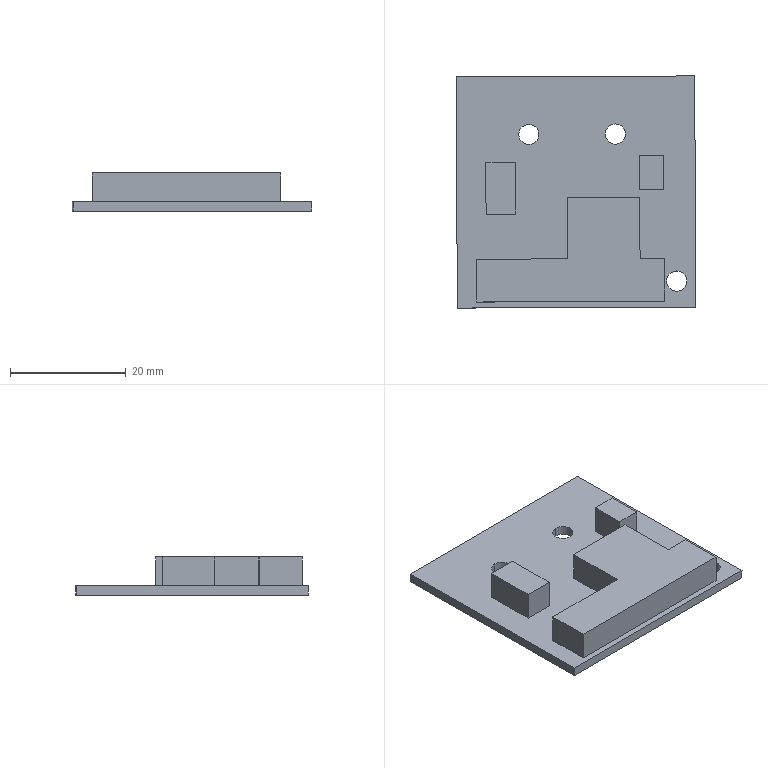Part | SolidWorks | features BaseBody 1 | 1 solid | 31 faces | box 41.444 x 40.179 x 6.6 mm | volume 4823 mm3 | plane 25 | cylinder 6 | commonest cylinder face diameters 3.5 x6
STEP:
#1=CARTESIAN_POINT('',(579.684,-227.507,-73.234));
#2=VERTEX_POINT('',#1);
#3=CARTESIAN_POINT('',(579.684,-224.007,-73.234));
#4=VERTEX_POINT('',#3);
#5=CARTESIAN_POINT('',(579.684,-225.757,-73.234));
#6=DIRECTION('',(-0.000000001,0.000000003,-1.));
#7=DIRECTION('',(0.,-1.,-0.000000003));
#8=AXIS2_PLACEMENT_3D('',#5,#6,#7);
#9=CIRCLE('',#8,1.75);
#10=EDGE_CURVE('',#2,#4,#9,.T.);
#11=ORIENTED_EDGE('',*,*,#10,.T.);
#12=CARTESIAN_POINT('',(579.684,-224.007,-71.634));
#13=VERTEX_POINT('',#12);
#14=CARTESIAN_POINT('',(579.684,-224.007,-73.234));
#15=DIRECTION('',(0.000000001,-0.000000003,1.));
#16=VECTOR('',#15,1000.);
#17=LINE('',#14,#16);
#18=EDGE_CURVE('',#4,#13,#17,.T.);
#19=ORIENTED_EDGE('',*,*,#18,.T.);
#20=CARTESIAN_POINT('',(579.684,-227.507,-71.634));
#21=VERTEX_POINT('',#20);
#22=CARTESIAN_POINT('',(579.684,-225.757,-71.634));
#23=DIRECTION('',(0.000000001,-0.000000003,1.));
#24=DIRECTION('',(0.,-1.,-0.000000003));
#25=AXIS2_PLACEMENT_3D('',#22,#23,#24);
#26=CIRCLE('',#25,1.75);
#27=EDGE_CURVE('',#13,#21,#26,.T.);
#28=ORIENTED_EDGE('',*,*,#27,.T.);
#29=CARTESIAN_POINT('',(579.684,-227.507,-73.234));
#30=DIRECTION('',(0.000000001,-0.000000003,1.));
#31=VECTOR('',#30,1000.);
#32=LINE('',#29,#31);
#33=EDGE_CURVE('',#2,#21,#32,.T.);
#34=ORIENTED_EDGE('',*,*,#33,.F.);
#35=EDGE_LOOP('',(#11,#19,#28,#34));
#36=FACE_OUTER_BOUND('',#35,.T.);
#37=CARTESIAN_POINT('',(579.684,-225.757,-73.234));
#38=DIRECTION('',(0.000000001,-0.000000003,1.));
#39=DIRECTION('',(0.,-1.,-0.000000003));
#40=AXIS2_PLACEMENT_3D('',#37,#38,#39);
#41=CYLINDRICAL_SURFACE('',#40,1.75);
#42=ADVANCED_FACE('',(#36),#41,.F.);
#43=CARTESIAN_POINT('',(569.073,-202.052,-73.234));
#44=VERTEX_POINT('',#43);
#45=CARTESIAN_POINT('',(569.073,-198.552,-73.234));
#46=VERTEX_POINT('',#45);
#47=CARTESIAN_POINT('',(569.073,-200.302,-73.234));
#48=DIRECTION('',(-0.000000001,0.000000003,-1.));
#49=DIRECTION('',(0.,-1.,-0.000000003));
#50=AXIS2_PLACEMENT_3D('',#47,#48,#49);
#51=CIRCLE('',#50,1.75);
#52=EDGE_CURVE('',#44,#46,#51,.T.);
#53=ORIENTED_EDGE('',*,*,#52,.T.);
#54=CARTESIAN_POINT('',(569.073,-198.552,-71.634));
#55=VERTEX_POINT('',#54);
#56=CARTESIAN_POINT('',(569.073,-198.552,-73.234));
#57=DIRECTION('',(0.000000001,-0.000000003,1.));
#58=VECTOR('',#57,1000.);
#59=LINE('',#56,#58);
#60=EDGE_CURVE('',#46,#55,#59,.T.);
#61=ORIENTED_EDGE('',*,*,#60,.T.);
#62=CARTESIAN_POINT('',(569.073,-202.052,-71.634));
#63=VERTEX_POINT('',#62);
#64=CARTESIAN_POINT('',(569.073,-200.302,-71.634));
#65=DIRECTION('',(0.000000001,-0.000000003,1.));
#66=DIRECTION('',(0.,-1.,-0.000000003));
#67=AXIS2_PLACEMENT_3D('',#64,#65,#66);
#68=CIRCLE('',#67,1.75);
#69=EDGE_CURVE('',#55,#63,#68,.T.);
#70=ORIENTED_EDGE('',*,*,#69,.T.);
#71=CARTESIAN_POINT('',(569.073,-202.052,-73.234));
#72=DIRECTION('',(0.000000001,-0.000000003,1.));
#73=VECTOR('',#72,1000.);
#74=LINE('',#71,#73);
#75=EDGE_CURVE('',#44,#63,#74,.T.);
#76=ORIENTED_EDGE('',*,*,#75,.F.);
#77=EDGE_LOOP('',(#53,#61,#70,#76));
#78=FACE_OUTER_BOUND('',#77,.T.);
#79=CARTESIAN_POINT('',(569.073,-200.302,-73.234));
#80=DIRECTION('',(0.000000001,-0.000000003,1.));
#81=DIRECTION('',(0.,-1.,-0.000000003));
#82=AXIS2_PLACEMENT_3D('',#79,#80,#81);
#83=CYLINDRICAL_SURFACE('',#82,1.75);
#84=ADVANCED_FACE('',(#78),#83,.F.);
#85=CARTESIAN_POINT('',(554.074,-202.118,-73.234));
#86=VERTEX_POINT('',#85);
#87=CARTESIAN_POINT('',(554.074,-198.618,-73.234));
#88=VERTEX_POINT('',#87);
#89=CARTESIAN_POINT('',(554.074,-200.368,-73.234));
#90=DIRECTION('',(-0.000000001,0.000000003,-1.));
#91=DIRECTION('',(0.,-1.,-0.000000003));
#92=AXIS2_PLACEMENT_3D('',#89,#90,#91);
#93=CIRCLE('',#92,1.75);
#94=EDGE_CURVE('',#86,#88,#93,.T.);
#95=ORIENTED_EDGE('',*,*,#94,.T.);
#96=CARTESIAN_POINT('',(554.074,-198.618,-71.634));
#97=VERTEX_POINT('',#96);
#98=CARTESIAN_POINT('',(554.074,-198.618,-73.234));
#99=DIRECTION('',(0.000000001,-0.000000003,1.));
#100=VECTOR('',#99,1000.);
#101=LINE('',#98,#100);
#102=EDGE_CURVE('',#88,#97,#101,.T.);
#103=ORIENTED_EDGE('',*,*,#102,.T.);
#104=CARTESIAN_POINT('',(554.074,-202.118,-71.634));
#105=VERTEX_POINT('',#104);
#106=CARTESIAN_POINT('',(554.074,-200.368,-71.634));
#107=DIRECTION('',(0.000000001,-0.000000003,1.));
#108=DIRECTION('',(0.,-1.,-0.000000003));
#109=AXIS2_PLACEMENT_3D('',#106,#107,#108);
#110=CIRCLE('',#109,1.75);
#111=EDGE_CURVE('',#97,#105,#110,.T.);
#112=ORIENTED_EDGE('',*,*,#111,.T.);
#113=CARTESIAN_POINT('',(554.074,-202.118,-73.234));
#114=DIRECTION('',(0.000000001,-0.000000003,1.));
#115=VECTOR('',#114,1000.);
#116=LINE('',#113,#115);
#117=EDGE_CURVE('',#86,#105,#116,.T.);
#118=ORIENTED_EDGE('',*,*,#117,.F.);
#119=EDGE_LOOP('',(#95,#103,#112,#118));
#120=FACE_OUTER_BOUND('',#119,.T.);
#121=CARTESIAN_POINT('',(554.074,-200.368,-73.234));
#122=DIRECTION('',(0.000000001,-0.000000003,1.));
#123=DIRECTION('',(0.,-1.,-0.000000003));
#124=AXIS2_PLACEMENT_3D('',#121,#122,#123);
#125=CYLINDRICAL_SURFACE('',#124,1.75);
#126=ADVANCED_FACE('',(#120),#125,.F.);
#127=ORIENTED_EDGE('',*,*,#10,.F.);
#128=CARTESIAN_POINT('',(579.684,-225.757,-73.234));
#129=DIRECTION('',(-0.000000001,0.000000003,-1.));
#130=DIRECTION('',(0.,-1.,-0.000000003));
#131=AXIS2_PLACEMENT_3D('',#128,#129,#130);
#132=CIRCLE('',#131,1.75);
#133=EDGE_CURVE('',#4,#2,#132,.T.);
#134=ORIENTED_EDGE('',*,*,#133,.F.);
#135=EDGE_LOOP('',(#127,#134));
#136=FACE_BOUND('',#135,.T.);
#137=ORIENTED_EDGE('',*,*,#52,.F.);
#138=CARTESIAN_POINT('',(569.073,-200.302,-73.234));
#139=DIRECTION('',(-0.000000001,0.000000003,-1.));
#140=DIRECTION('',(0.,-1.,-0.000000003));
#141=AXIS2_PLACEMENT_3D('',#138,#139,#140);
#142=CIRCLE('',#141,1.75);
#143=EDGE_CURVE('',#46,#44,#142,.T.);
#144=ORIENTED_EDGE('',*,*,#143,.F.);
#145=EDGE_LOOP('',(#137,#144));
#146=FACE_BOUND('',#145,.T.);
#147=ORIENTED_EDGE('',*,*,#94,.F.);
#148=CARTESIAN_POINT('',(554.074,-200.368,-73.234));
#149=DIRECTION('',(-0.000000001,0.000000003,-1.));
#150=DIRECTION('',(0.,-1.,-0.000000003));
#151=AXIS2_PLACEMENT_3D('',#148,#149,#150);
#152=CIRCLE('',#151,1.75);
#153=EDGE_CURVE('',#88,#86,#152,.T.);
#154=ORIENTED_EDGE('',*,*,#153,.F.);
#155=EDGE_LOOP('',(#147,#154));
#156=FACE_BOUND('',#155,.T.);
#157=CARTESIAN_POINT('',(582.974,-230.242,-73.234));
#158=VERTEX_POINT('',#157);
#159=CARTESIAN_POINT('',(582.8,-190.243,-73.234));
#160=VERTEX_POINT('',#159);
#161=CARTESIAN_POINT('',(582.887,-210.242,-73.234));
#162=DIRECTION('',(-0.004352,1.,0.000000003));
#163=VECTOR('',#162,1000.);
#164=LINE('',#161,#163);
#165=EDGE_CURVE('',#158,#160,#164,.T.);
#166=ORIENTED_EDGE('',*,*,#165,.F.);
#167=CARTESIAN_POINT('',(541.704,-230.422,-73.234));
#168=VERTEX_POINT('',#167);
#169=CARTESIAN_POINT('',(562.339,-230.332,-73.234));
#170=DIRECTION('',(1.,0.004352,-0.000000001));
#171=VECTOR('',#170,1000.);
#172=LINE('',#169,#171);
#173=EDGE_CURVE('',#168,#158,#172,.T.);
#174=ORIENTED_EDGE('',*,*,#173,.F.);
#175=CARTESIAN_POINT('',(541.53,-190.422,-73.234));
#176=VERTEX_POINT('',#175);
#177=CARTESIAN_POINT('',(541.617,-210.422,-73.234));
#178=DIRECTION('',(0.004352,-1.,-0.000000003));
#179=VECTOR('',#178,1000.);
#180=LINE('',#177,#179);
#181=EDGE_CURVE('',#176,#168,#180,.T.);
#182=ORIENTED_EDGE('',*,*,#181,.F.);
#183=CARTESIAN_POINT('',(562.165,-190.332,-73.234));
#184=DIRECTION('',(-1.,-0.004352,0.000000001));
#185=VECTOR('',#184,1000.);
#186=LINE('',#183,#185);
#187=EDGE_CURVE('',#160,#176,#186,.T.);
#188=ORIENTED_EDGE('',*,*,#187,.F.);
#189=EDGE_LOOP('',(#166,#174,#182,#188));
#190=FACE_OUTER_BOUND('',#189,.T.);
#191=CARTESIAN_POINT('',(540.701,-189.626,-73.234));
#192=DIRECTION('',(0.000000001,-0.000000003,1.));
#193=DIRECTION('',(0.004352,-1.,-0.000000003));
#194=AXIS2_PLACEMENT_3D('',#191,#192,#193);
#195=PLANE('',#194);
#196=ADVANCED_FACE('',(#136,#146,#156,#190),#195,.F.);
#197=ORIENTED_EDGE('',*,*,#18,.F.);
#198=ORIENTED_EDGE('',*,*,#133,.T.);
#199=ORIENTED_EDGE('',*,*,#33,.T.);
#200=CARTESIAN_POINT('',(579.684,-225.757,-71.634));
#201=DIRECTION('',(0.000000001,-0.000000003,1.));
#202=DIRECTION('',(0.,-1.,-0.000000003));
#203=AXIS2_PLACEMENT_3D('',#200,#201,#202);
#204=CIRCLE('',#203,1.75);
#205=EDGE_CURVE('',#21,#13,#204,.T.);
#206=ORIENTED_EDGE('',*,*,#205,.T.);
#207=EDGE_LOOP('',(#197,#198,#199,#206));
#208=FACE_OUTER_BOUND('',#207,.T.);
#209=CARTESIAN_POINT('',(579.684,-225.757,-73.234));
#210=DIRECTION('',(0.000000001,-0.000000003,1.));
#211=DIRECTION('',(0.,-1.,-0.000000003));
#212=AXIS2_PLACEMENT_3D('',#209,#210,#211);
#213=CYLINDRICAL_SURFACE('',#212,1.75);
#214=ADVANCED_FACE('',(#208),#213,.F.);
#215=ORIENTED_EDGE('',*,*,#60,.F.);
#216=ORIENTED_EDGE('',*,*,#143,.T.);
#217=ORIENTED_EDGE('',*,*,#75,.T.);
#218=CARTESIAN_POINT('',(569.073,-200.302,-71.634));
#219=DIRECTION('',(0.000000001,-0.000000003,1.));
#220=DIRECTION('',(0.,-1.,-0.000000003));
#221=AXIS2_PLACEMENT_3D('',#218,#219,#220);
#222=CIRCLE('',#221,1.75);
#223=EDGE_CURVE('',#63,#55,#222,.T.);
#224=ORIENTED_EDGE('',*,*,#223,.T.);
#225=EDGE_LOOP('',(#215,#216,#217,#224));
#226=FACE_OUTER_BOUND('',#225,.T.);
#227=CARTESIAN_POINT('',(569.073,-200.302,-73.234));
#228=DIRECTION('',(0.000000001,-0.000000003,1.));
#229=DIRECTION('',(0.,-1.,-0.000000003));
#230=AXIS2_PLACEMENT_3D('',#227,#228,#229);
#231=CYLINDRICAL_SURFACE('',#230,1.75);
#232=ADVANCED_FACE('',(#226),#231,.F.);
#233=ORIENTED_EDGE('',*,*,#102,.F.);
#234=ORIENTED_EDGE('',*,*,#153,.T.);
#235=ORIENTED_EDGE('',*,*,#117,.T.);
#236=CARTESIAN_POINT('',(554.074,-200.368,-71.634));
#237=DIRECTION('',(0.000000001,-0.000000003,1.));
#238=DIRECTION('',(0.,-1.,-0.000000003));
#239=AXIS2_PLACEMENT_3D('',#236,#237,#238);
#240=CIRCLE('',#239,1.75);
#241=EDGE_CURVE('',#105,#97,#240,.T.);
#242=ORIENTED_EDGE('',*,*,#241,.T.);
#243=EDGE_LOOP('',(#233,#234,#235,#242));
#244=FACE_OUTER_BOUND('',#243,.T.);
#245=CARTESIAN_POINT('',(554.074,-200.368,-73.234));
#246=DIRECTION('',(0.000000001,-0.000000003,1.));
#247=DIRECTION('',(0.,-1.,-0.000000003));
#248=AXIS2_PLACEMENT_3D('',#245,#246,#247);
#249=CYLINDRICAL_SURFACE('',#248,1.75);
#250=ADVANCED_FACE('',(#244),#249,.F.);
#251=CARTESIAN_POINT('',(541.53,-190.422,-71.634));
#252=VERTEX_POINT('',#251);
#253=CARTESIAN_POINT('',(582.8,-190.243,-71.634));
#254=VERTEX_POINT('',#253);
#255=CARTESIAN_POINT('',(562.165,-190.332,-71.634));
#256=DIRECTION('',(1.,0.004352,-0.000000001));
#257=VECTOR('',#256,1000.);
#258=LINE('',#255,#257);
#259=EDGE_CURVE('',#252,#254,#258,.T.);
#260=ORIENTED_EDGE('',*,*,#259,.T.);
#261=CARTESIAN_POINT('',(582.8,-190.243,-72.434));
#262=DIRECTION('',(-0.000000001,0.000000003,-1.));
#263=VECTOR('',#262,1000.);
#264=LINE('',#261,#263);
#265=EDGE_CURVE('',#254,#160,#264,.T.);
#266=ORIENTED_EDGE('',*,*,#265,.T.);
#267=ORIENTED_EDGE('',*,*,#187,.T.);
#268=CARTESIAN_POINT('',(541.53,-190.422,-72.434));
#269=DIRECTION('',(0.000000001,-0.000000003,1.));
#270=VECTOR('',#269,1000.);
#271=LINE('',#268,#270);
#272=EDGE_CURVE('',#176,#252,#271,.T.);
#273=ORIENTED_EDGE('',*,*,#272,.T.);
#274=EDGE_LOOP('',(#260,#266,#267,#273));
#275=FACE_OUTER_BOUND('',#274,.T.);
#276=CARTESIAN_POINT('',(583.625,-190.239,-73.266));
#277=DIRECTION('',(-0.004352,1.,0.000000003));
#278=DIRECTION('',(-1.,-0.004352,0.000000001));
#279=AXIS2_PLACEMENT_3D('',#276,#277,#278);
#280=PLANE('',#279);
#281=ADVANCED_FACE('',(#275),#280,.T.);
#282=CARTESIAN_POINT('',(582.974,-230.242,-71.634));
#283=VERTEX_POINT('',#282);
#284=CARTESIAN_POINT('',(582.887,-210.242,-71.634));
#285=DIRECTION('',(0.004352,-1.,-0.000000003));
#286=VECTOR('',#285,1000.);
#287=LINE('',#284,#286);
#288=EDGE_CURVE('',#254,#283,#287,.T.);
#289=ORIENTED_EDGE('',*,*,#288,.T.);
#290=CARTESIAN_POINT('',(582.974,-230.242,-72.434));
#291=DIRECTION('',(-0.000000001,0.000000003,-1.));
#292=VECTOR('',#291,1000.);
#293=LINE('',#290,#292);
#294=EDGE_CURVE('',#283,#158,#293,.T.);
#295=ORIENTED_EDGE('',*,*,#294,.T.);
#296=ORIENTED_EDGE('',*,*,#165,.T.);
#297=ORIENTED_EDGE('',*,*,#265,.F.);
#298=EDGE_LOOP('',(#289,#295,#296,#297));
#299=FACE_OUTER_BOUND('',#298,.T.);
#300=CARTESIAN_POINT('',(582.977,-231.042,-73.266));
#301=DIRECTION('',(1.,0.004352,-0.000000001));
#302=DIRECTION('',(-0.004352,1.,0.000000003));
#303=AXIS2_PLACEMENT_3D('',#300,#301,#302);
#304=PLANE('',#303);
#305=ADVANCED_FACE('',(#299),#304,.T.);
#306=CARTESIAN_POINT('',(541.704,-230.422,-71.634));
#307=VERTEX_POINT('',#306);
#308=CARTESIAN_POINT('',(562.339,-230.332,-71.634));
#309=DIRECTION('',(-1.,-0.004352,0.000000001));
#310=VECTOR('',#309,1000.);
#311=LINE('',#308,#310);
#312=EDGE_CURVE('',#283,#307,#311,.T.);
#313=ORIENTED_EDGE('',*,*,#312,.T.);
#314=CARTESIAN_POINT('',(541.704,-230.422,-72.434));
#315=DIRECTION('',(-0.000000001,0.000000003,-1.));
#316=VECTOR('',#315,1000.);
#317=LINE('',#314,#316);
#318=EDGE_CURVE('',#307,#168,#317,.T.);
#319=ORIENTED_EDGE('',*,*,#318,.T.);
#320=ORIENTED_EDGE('',*,*,#173,.T.);
#321=ORIENTED_EDGE('',*,*,#294,.F.);
#322=EDGE_LOOP('',(#313,#319,#320,#321));
#323=FACE_OUTER_BOUND('',#322,.T.);
#324=CARTESIAN_POINT('',(540.879,-230.425,-73.266));
#325=DIRECTION('',(0.004352,-1.,-0.000000003));
#326=DIRECTION('',(1.,0.004352,-0.000000001));
#327=AXIS2_PLACEMENT_3D('',#324,#325,#326);
#328=PLANE('',#327);
#329=ADVANCED_FACE('',(#323),#328,.T.);
#330=CARTESIAN_POINT('',(541.617,-210.422,-71.634));
#331=DIRECTION('',(-0.004352,1.,0.000000003));
#332=VECTOR('',#331,1000.);
#333=LINE('',#330,#332);
#334=EDGE_CURVE('',#307,#252,#333,.T.);
#335=ORIENTED_EDGE('',*,*,#334,.T.);
#336=ORIENTED_EDGE('',*,*,#272,.F.);
#337=ORIENTED_EDGE('',*,*,#181,.T.);
#338=ORIENTED_EDGE('',*,*,#318,.F.);
#339=EDGE_LOOP('',(#335,#336,#337,#338));
#340=FACE_OUTER_BOUND('',#339,.T.);
#341=CARTESIAN_POINT('',(541.527,-189.622,-73.266));
#342=DIRECTION('',(-1.,-0.004352,0.000000001));
#343=DIRECTION('',(0.004352,-1.,-0.000000003));
#344=AXIS2_PLACEMENT_3D('',#341,#342,#343);
#345=PLANE('',#344);
#346=ADVANCED_FACE('',(#340),#345,.T.);
#347=CARTESIAN_POINT('',(577.45,-209.957,-71.634));
#348=VERTEX_POINT('',#347);
#349=CARTESIAN_POINT('',(573.284,-209.976,-71.634));
#350=VERTEX_POINT('',#349);
#351=CARTESIAN_POINT('',(562.251,-210.024,-71.634));
#352=DIRECTION('',(-1.,-0.004352,0.000000001));
#353=VECTOR('',#352,1000.);
#354=LINE('',#351,#353);
#355=EDGE_CURVE('',#348,#350,#354,.T.);
#356=ORIENTED_EDGE('',*,*,#355,.T.);
#357=CARTESIAN_POINT('',(573.258,-204.035,-71.634));
#358=VERTEX_POINT('',#357);
#359=CARTESIAN_POINT('',(573.285,-210.284,-71.634));
#360=DIRECTION('',(-0.004352,1.,0.000000003));
#361=VECTOR('',#360,1000.);
#362=LINE('',#359,#361);
#363=EDGE_CURVE('',#350,#358,#362,.T.);
#364=ORIENTED_EDGE('',*,*,#363,.T.);
#365=CARTESIAN_POINT('',(577.424,-204.017,-71.634));
#366=VERTEX_POINT('',#365);
#367=CARTESIAN_POINT('',(562.225,-204.083,-71.634));
#368=DIRECTION('',(1.,0.004352,-0.000000001));
#369=VECTOR('',#368,1000.);
#370=LINE('',#367,#369);
#371=EDGE_CURVE('',#358,#366,#370,.T.);
#372=ORIENTED_EDGE('',*,*,#371,.T.);
#373=CARTESIAN_POINT('',(577.451,-210.266,-71.634));
#374=DIRECTION('',(0.004352,-1.,-0.000000003));
#375=VECTOR('',#374,1000.);
#376=LINE('',#373,#375);
#377=EDGE_CURVE('',#366,#348,#376,.T.);
#378=ORIENTED_EDGE('',*,*,#377,.T.);
#379=EDGE_LOOP('',(#356,#364,#372,#378));
#380=FACE_BOUND('',#379,.T.);
#381=CARTESIAN_POINT('',(551.853,-214.158,-71.634));
#382=VERTEX_POINT('',#381);
#383=CARTESIAN_POINT('',(546.683,-214.181,-71.634));
#384=VERTEX_POINT('',#383);
#385=CARTESIAN_POINT('',(562.269,-214.113,-71.634));
#386=DIRECTION('',(-1.,-0.004352,0.000000001));
#387=VECTOR('',#386,1000.);
#388=LINE('',#385,#387);
#389=EDGE_CURVE('',#382,#384,#388,.T.);
#390=ORIENTED_EDGE('',*,*,#389,.T.);
#391=CARTESIAN_POINT('',(546.645,-205.231,-71.634));
#392=VERTEX_POINT('',#391);
#393=CARTESIAN_POINT('',(546.667,-210.4,-71.634));
#394=DIRECTION('',(-0.004352,1.,0.000000003));
#395=VECTOR('',#394,1000.);
#396=LINE('',#393,#395);
#397=EDGE_CURVE('',#384,#392,#396,.T.);
#398=ORIENTED_EDGE('',*,*,#397,.T.);
#399=CARTESIAN_POINT('',(551.814,-205.208,-71.634));
#400=VERTEX_POINT('',#399);
#401=CARTESIAN_POINT('',(562.23,-205.163,-71.634));
#402=DIRECTION('',(1.,0.004352,-0.000000001));
#403=VECTOR('',#402,1000.);
#404=LINE('',#401,#403);
#405=EDGE_CURVE('',#392,#400,#404,.T.);
#406=ORIENTED_EDGE('',*,*,#405,.T.);
#407=CARTESIAN_POINT('',(551.836,-210.378,-71.634));
#408=DIRECTION('',(0.004352,-1.,-0.000000003));
#409=VECTOR('',#408,1000.);
#410=LINE('',#407,#409);
#411=EDGE_CURVE('',#400,#382,#410,.T.);
#412=ORIENTED_EDGE('',*,*,#411,.T.);
#413=EDGE_LOOP('',(#390,#398,#406,#412));
#414=FACE_BOUND('',#413,.T.);
#415=CARTESIAN_POINT('',(544.944,-221.98,-71.634));
#416=VERTEX_POINT('',#415);
#417=CARTESIAN_POINT('',(560.759,-221.911,-71.634));
#418=VERTEX_POINT('',#417);
#419=CARTESIAN_POINT('',(562.302,-221.904,-71.634));
#420=DIRECTION('',(1.,0.004352,-0.000000001));
#421=VECTOR('',#420,1000.);
#422=LINE('',#419,#421);
#423=EDGE_CURVE('',#416,#418,#422,.T.);
#424=ORIENTED_EDGE('',*,*,#423,.T.);
#425=CARTESIAN_POINT('',(560.713,-211.342,-71.634));
#426=VERTEX_POINT('',#425);
#427=CARTESIAN_POINT('',(560.709,-210.339,-71.634));
#428=DIRECTION('',(-0.004352,1.,0.000000003));
#429=VECTOR('',#428,1000.);
#430=LINE('',#427,#429);
#431=EDGE_CURVE('',#418,#426,#430,.T.);
#432=ORIENTED_EDGE('',*,*,#431,.T.);
#433=CARTESIAN_POINT('',(573.289,-211.287,-71.634));
#434=VERTEX_POINT('',#433);
#435=CARTESIAN_POINT('',(562.256,-211.335,-71.634));
#436=DIRECTION('',(1.,0.004352,-0.000000001));
#437=VECTOR('',#436,1000.);
#438=LINE('',#435,#437);
#439=EDGE_CURVE('',#426,#434,#438,.T.);
#440=ORIENTED_EDGE('',*,*,#439,.T.);
#441=CARTESIAN_POINT('',(573.335,-221.856,-71.634));
#442=VERTEX_POINT('',#441);
#443=CARTESIAN_POINT('',(573.285,-210.284,-71.634));
#444=DIRECTION('',(0.004352,-1.,-0.000000003));
#445=VECTOR('',#444,1000.);
#446=LINE('',#443,#445);
#447=EDGE_CURVE('',#434,#442,#446,.T.);
#448=ORIENTED_EDGE('',*,*,#447,.T.);
#449=CARTESIAN_POINT('',(577.578,-221.838,-71.634));
#450=VERTEX_POINT('',#449);
#451=CARTESIAN_POINT('',(562.302,-221.904,-71.634));
#452=DIRECTION('',(1.,0.004352,-0.000000001));
#453=VECTOR('',#452,1000.);
#454=LINE('',#451,#453);
#455=EDGE_CURVE('',#442,#450,#454,.T.);
#456=ORIENTED_EDGE('',*,*,#455,.T.);
#457=CARTESIAN_POINT('',(577.61,-229.244,-71.634));
#458=VERTEX_POINT('',#457);
#459=CARTESIAN_POINT('',(577.527,-210.266,-71.634));
#460=DIRECTION('',(0.004352,-1.,-0.000000003));
#461=VECTOR('',#460,1000.);
#462=LINE('',#459,#461);
#463=EDGE_CURVE('',#450,#458,#462,.T.);
#464=ORIENTED_EDGE('',*,*,#463,.T.);
#465=CARTESIAN_POINT('',(544.977,-229.386,-71.634));
#466=VERTEX_POINT('',#465);
#467=CARTESIAN_POINT('',(562.335,-229.31,-71.634));
#468=DIRECTION('',(-1.,-0.004352,0.000000001));
#469=VECTOR('',#468,1000.);
#470=LINE('',#467,#469);
#471=EDGE_CURVE('',#458,#466,#470,.T.);
#472=ORIENTED_EDGE('',*,*,#471,.T.);
#473=CARTESIAN_POINT('',(544.894,-210.408,-71.634));
#474=DIRECTION('',(-0.004352,1.,0.000000003));
#475=VECTOR('',#474,1000.);
#476=LINE('',#473,#475);
#477=EDGE_CURVE('',#466,#416,#476,.T.);
#478=ORIENTED_EDGE('',*,*,#477,.T.);
#479=EDGE_LOOP('',(#424,#432,#440,#448,#456,#464,#472,#478));
#480=FACE_BOUND('',#479,.T.);
#481=ORIENTED_EDGE('',*,*,#205,.F.);
#482=ORIENTED_EDGE('',*,*,#27,.F.);
#483=EDGE_LOOP('',(#481,#482));
#484=FACE_BOUND('',#483,.T.);
#485=ORIENTED_EDGE('',*,*,#223,.F.);
#486=ORIENTED_EDGE('',*,*,#69,.F.);
#487=EDGE_LOOP('',(#485,#486));
#488=FACE_BOUND('',#487,.T.);
#489=ORIENTED_EDGE('',*,*,#241,.F.);
#490=ORIENTED_EDGE('',*,*,#111,.F.);
#491=EDGE_LOOP('',(#489,#490));
#492=FACE_BOUND('',#491,.T.);
#493=ORIENTED_EDGE('',*,*,#312,.F.);
#494=ORIENTED_EDGE('',*,*,#288,.F.);
#495=ORIENTED_EDGE('',*,*,#259,.F.);
#496=ORIENTED_EDGE('',*,*,#334,.F.);
#497=EDGE_LOOP('',(#493,#494,#495,#496));
#498=FACE_OUTER_BOUND('',#497,.T.);
#499=CARTESIAN_POINT('',(540.701,-189.626,-71.634));
#500=DIRECTION('',(0.000000001,-0.000000003,1.));
#501=DIRECTION('',(0.004352,-1.,-0.000000003));
#502=AXIS2_PLACEMENT_3D('',#499,#500,#501);
#503=PLANE('',#502);
#504=ADVANCED_FACE('',(#380,#414,#480,#484,#488,#492,#498),#503,.T.);
#505=CARTESIAN_POINT('',(573.284,-209.976,-66.634));
#506=VERTEX_POINT('',#505);
#507=CARTESIAN_POINT('',(573.258,-204.035,-66.634));
#508=VERTEX_POINT('',#507);
#509=CARTESIAN_POINT('',(573.271,-207.005,-66.634));
#510=DIRECTION('',(-0.004352,1.,0.000000003));
#511=VECTOR('',#510,1000.);
#512=LINE('',#509,#511);
#513=EDGE_CURVE('',#506,#508,#512,.T.);
#514=ORIENTED_EDGE('',*,*,#513,.T.);
#515=CARTESIAN_POINT('',(573.258,-204.035,-69.134));
#516=DIRECTION('',(-0.000000001,0.000000003,-1.));
#517=VECTOR('',#516,1000.);
#518=LINE('',#515,#517);
#519=EDGE_CURVE('',#508,#358,#518,.T.);
#520=ORIENTED_EDGE('',*,*,#519,.T.);
#521=ORIENTED_EDGE('',*,*,#363,.F.);
#522=CARTESIAN_POINT('',(573.284,-209.976,-69.134));
#523=DIRECTION('',(0.000000001,-0.000000003,1.));
#524=VECTOR('',#523,1000.);
#525=LINE('',#522,#524);
#526=EDGE_CURVE('',#350,#506,#525,.T.);
#527=ORIENTED_EDGE('',*,*,#526,.T.);
#528=EDGE_LOOP('',(#514,#520,#521,#527));
#529=FACE_OUTER_BOUND('',#528,.T.);
#530=CARTESIAN_POINT('',(573.257,-203.916,-71.734));
#531=DIRECTION('',(-1.,-0.004352,0.000000001));
#532=DIRECTION('',(0.004352,-1.,-0.000000003));
#533=AXIS2_PLACEMENT_3D('',#530,#531,#532);
#534=PLANE('',#533);
#535=ADVANCED_FACE('',(#529),#534,.T.);
#536=CARTESIAN_POINT('',(577.45,-209.957,-66.634));
#537=VERTEX_POINT('',#536);
#538=CARTESIAN_POINT('',(575.367,-209.967,-66.634));
#539=DIRECTION('',(-1.,-0.004352,0.000000001));
#540=VECTOR('',#539,1000.);
#541=LINE('',#538,#540);
#542=EDGE_CURVE('',#537,#506,#541,.T.);
#543=ORIENTED_EDGE('',*,*,#542,.T.);
#544=ORIENTED_EDGE('',*,*,#526,.F.);
#545=ORIENTED_EDGE('',*,*,#355,.F.);
#546=CARTESIAN_POINT('',(577.45,-209.957,-69.134));
#547=DIRECTION('',(0.000000001,-0.000000003,1.));
#548=VECTOR('',#547,1000.);
#549=LINE('',#546,#548);
#550=EDGE_CURVE('',#348,#537,#549,.T.);
#551=ORIENTED_EDGE('',*,*,#550,.T.);
#552=EDGE_LOOP('',(#543,#544,#545,#551));
#553=FACE_OUTER_BOUND('',#552,.T.);
#554=CARTESIAN_POINT('',(573.2,-209.976,-71.734));
#555=DIRECTION('',(0.004352,-1.,-0.000000003));
#556=DIRECTION('',(1.,0.004352,-0.000000001));
#557=AXIS2_PLACEMENT_3D('',#554,#555,#556);
#558=PLANE('',#557);
#559=ADVANCED_FACE('',(#553),#558,.T.);
#560=CARTESIAN_POINT('',(577.424,-204.017,-66.634));
#561=VERTEX_POINT('',#560);
#562=CARTESIAN_POINT('',(577.437,-206.987,-66.634));
#563=DIRECTION('',(0.004352,-1.,-0.000000003));
#564=VECTOR('',#563,1000.);
#565=LINE('',#562,#564);
#566=EDGE_CURVE('',#561,#537,#565,.T.);
#567=ORIENTED_EDGE('',*,*,#566,.T.);
#568=ORIENTED_EDGE('',*,*,#550,.F.);
#569=ORIENTED_EDGE('',*,*,#377,.F.);
#570=CARTESIAN_POINT('',(577.424,-204.017,-69.134));
#571=DIRECTION('',(0.000000001,-0.000000003,1.));
#572=VECTOR('',#571,1000.);
#573=LINE('',#570,#572);
#574=EDGE_CURVE('',#366,#561,#573,.T.);
#575=ORIENTED_EDGE('',*,*,#574,.T.);
#576=EDGE_LOOP('',(#567,#568,#569,#575));
#577=FACE_OUTER_BOUND('',#576,.T.);
#578=CARTESIAN_POINT('',(577.451,-210.076,-71.734));
#579=DIRECTION('',(1.,0.004352,-0.000000001));
#580=DIRECTION('',(-0.004352,1.,0.000000003));
#581=AXIS2_PLACEMENT_3D('',#578,#579,#580);
#582=PLANE('',#581);
#583=ADVANCED_FACE('',(#577),#582,.T.);
#584=CARTESIAN_POINT('',(575.341,-204.026,-66.634));
#585=DIRECTION('',(1.,0.004352,-0.000000001));
#586=VECTOR('',#585,1000.);
#587=LINE('',#584,#586);
#588=EDGE_CURVE('',#508,#561,#587,.T.);
#589=ORIENTED_EDGE('',*,*,#588,.T.);
#590=ORIENTED_EDGE('',*,*,#574,.F.);
#591=ORIENTED_EDGE('',*,*,#371,.F.);
#592=ORIENTED_EDGE('',*,*,#519,.F.);
#593=EDGE_LOOP('',(#589,#590,#591,#592));
#594=FACE_OUTER_BOUND('',#593,.T.);
#595=CARTESIAN_POINT('',(577.507,-204.016,-71.734));
#596=DIRECTION('',(-0.004352,1.,0.000000003));
#597=DIRECTION('',(-1.,-0.004352,0.000000001));
#598=AXIS2_PLACEMENT_3D('',#595,#596,#597);
#599=PLANE('',#598);
#600=ADVANCED_FACE('',(#594),#599,.T.);
#601=CARTESIAN_POINT('',(546.683,-214.181,-66.634));
#602=VERTEX_POINT('',#601);
#603=CARTESIAN_POINT('',(546.645,-205.231,-66.634));
#604=VERTEX_POINT('',#603);
#605=CARTESIAN_POINT('',(546.664,-209.706,-66.634));
#606=DIRECTION('',(-0.004352,1.,0.000000003));
#607=VECTOR('',#606,1000.);
#608=LINE('',#605,#607);
#609=EDGE_CURVE('',#602,#604,#608,.T.);
#610=ORIENTED_EDGE('',*,*,#609,.T.);
#611=CARTESIAN_POINT('',(546.645,-205.231,-69.134));
#612=DIRECTION('',(-0.000000001,0.000000003,-1.));
#613=VECTOR('',#612,1000.);
#614=LINE('',#611,#613);
#615=EDGE_CURVE('',#604,#392,#614,.T.);
#616=ORIENTED_EDGE('',*,*,#615,.T.);
#617=ORIENTED_EDGE('',*,*,#397,.F.);
#618=CARTESIAN_POINT('',(546.683,-214.181,-69.134));
#619=DIRECTION('',(0.000000001,-0.000000003,1.));
#620=VECTOR('',#619,1000.);
#621=LINE('',#618,#620);
#622=EDGE_CURVE('',#384,#602,#621,.T.);
#623=ORIENTED_EDGE('',*,*,#622,.T.);
#624=EDGE_LOOP('',(#610,#616,#617,#623));
#625=FACE_OUTER_BOUND('',#624,.T.);
#626=CARTESIAN_POINT('',(546.644,-205.052,-71.734));
#627=DIRECTION('',(-1.,-0.004352,0.000000001));
#628=DIRECTION('',(0.004352,-1.,-0.000000003));
#629=AXIS2_PLACEMENT_3D('',#626,#627,#628);
#630=PLANE('',#629);
#631=ADVANCED_FACE('',(#625),#630,.T.);
#632=CARTESIAN_POINT('',(551.853,-214.158,-66.634));
#633=VERTEX_POINT('',#632);
#634=CARTESIAN_POINT('',(549.268,-214.169,-66.634));
#635=DIRECTION('',(-1.,-0.004352,0.000000001));
#636=VECTOR('',#635,1000.);
#637=LINE('',#634,#636);
#638=EDGE_CURVE('',#633,#602,#637,.T.);
#639=ORIENTED_EDGE('',*,*,#638,.T.);
#640=ORIENTED_EDGE('',*,*,#622,.F.);
#641=ORIENTED_EDGE('',*,*,#389,.F.);
#642=CARTESIAN_POINT('',(551.853,-214.158,-69.134));
#643=DIRECTION('',(0.000000001,-0.000000003,1.));
#644=VECTOR('',#643,1000.);
#645=LINE('',#642,#644);
#646=EDGE_CURVE('',#382,#633,#645,.T.);
#647=ORIENTED_EDGE('',*,*,#646,.T.);
#648=EDGE_LOOP('',(#639,#640,#641,#647));
#649=FACE_OUTER_BOUND('',#648,.T.);
#650=CARTESIAN_POINT('',(546.58,-214.181,-71.734));
#651=DIRECTION('',(0.004352,-1.,-0.000000003));
#652=DIRECTION('',(1.,0.004352,-0.000000001));
#653=AXIS2_PLACEMENT_3D('',#650,#651,#652);
#654=PLANE('',#653);
#655=ADVANCED_FACE('',(#649),#654,.T.);
#656=CARTESIAN_POINT('',(551.814,-205.208,-66.634));
#657=VERTEX_POINT('',#656);
#658=CARTESIAN_POINT('',(551.833,-209.683,-66.634));
#659=DIRECTION('',(0.004352,-1.,-0.000000003));
#660=VECTOR('',#659,1000.);
#661=LINE('',#658,#660);
#662=EDGE_CURVE('',#657,#633,#661,.T.);
#663=ORIENTED_EDGE('',*,*,#662,.T.);
#664=ORIENTED_EDGE('',*,*,#646,.F.);
#665=ORIENTED_EDGE('',*,*,#411,.F.);
#666=CARTESIAN_POINT('',(551.814,-205.208,-69.134));
#667=DIRECTION('',(0.000000001,-0.000000003,1.));
#668=VECTOR('',#667,1000.);
#669=LINE('',#666,#668);
#670=EDGE_CURVE('',#400,#657,#669,.T.);
#671=ORIENTED_EDGE('',*,*,#670,.T.);
#672=EDGE_LOOP('',(#663,#664,#665,#671));
#673=FACE_OUTER_BOUND('',#672,.T.);
#674=CARTESIAN_POINT('',(551.854,-214.337,-71.734));
#675=DIRECTION('',(1.,0.004352,-0.000000001));
#676=DIRECTION('',(-0.004352,1.,0.000000003));
#677=AXIS2_PLACEMENT_3D('',#674,#675,#676);
#678=PLANE('',#677);
#679=ADVANCED_FACE('',(#673),#678,.T.);
#680=CARTESIAN_POINT('',(549.229,-205.22,-66.634));
#681=DIRECTION('',(1.,0.004352,-0.000000001));
#682=VECTOR('',#681,1000.);
#683=LINE('',#680,#682);
#684=EDGE_CURVE('',#604,#657,#683,.T.);
#685=ORIENTED_EDGE('',*,*,#684,.T.);
#686=ORIENTED_EDGE('',*,*,#670,.F.);
#687=ORIENTED_EDGE('',*,*,#405,.F.);
#688=ORIENTED_EDGE('',*,*,#615,.F.);
#689=EDGE_LOOP('',(#685,#686,#687,#688));
#690=FACE_OUTER_BOUND('',#689,.T.);
#691=CARTESIAN_POINT('',(551.917,-205.208,-71.734));
#692=DIRECTION('',(-0.004352,1.,0.000000003));
#693=DIRECTION('',(-1.,-0.004352,0.000000001));
#694=AXIS2_PLACEMENT_3D('',#691,#692,#693);
#695=PLANE('',#694);
#696=ADVANCED_FACE('',(#690),#695,.T.);
#697=CARTESIAN_POINT('',(560.759,-221.911,-66.634));
#698=VERTEX_POINT('',#697);
#699=CARTESIAN_POINT('',(560.713,-211.342,-66.634));
#700=VERTEX_POINT('',#699);
#701=CARTESIAN_POINT('',(560.736,-216.627,-66.634));
#702=DIRECTION('',(-0.004352,1.,0.000000003));
#703=VECTOR('',#702,1000.);
#704=LINE('',#701,#703);
#705=EDGE_CURVE('',#698,#700,#704,.T.);
#706=ORIENTED_EDGE('',*,*,#705,.T.);
#707=CARTESIAN_POINT('',(560.713,-211.342,-69.134));
#708=DIRECTION('',(-0.000000001,0.000000003,-1.));
#709=VECTOR('',#708,1000.);
#710=LINE('',#707,#709);
#711=EDGE_CURVE('',#700,#426,#710,.T.);
#712=ORIENTED_EDGE('',*,*,#711,.T.);
#713=ORIENTED_EDGE('',*,*,#431,.F.);
#714=CARTESIAN_POINT('',(560.759,-221.911,-69.134));
#715=DIRECTION('',(0.000000001,-0.000000003,1.));
#716=VECTOR('',#715,1000.);
#717=LINE('',#714,#716);
#718=EDGE_CURVE('',#418,#698,#717,.T.);
#719=ORIENTED_EDGE('',*,*,#718,.T.);
#720=EDGE_LOOP('',(#706,#712,#713,#719));
#721=FACE_OUTER_BOUND('',#720,.T.);
#722=CARTESIAN_POINT('',(560.712,-211.131,-71.734));
#723=DIRECTION('',(-1.,-0.004352,0.000000001));
#724=DIRECTION('',(0.004352,-1.,-0.000000003));
#725=AXIS2_PLACEMENT_3D('',#722,#723,#724);
#726=PLANE('',#725);
#727=ADVANCED_FACE('',(#721),#726,.T.);
#728=CARTESIAN_POINT('',(544.944,-221.98,-66.634));
#729=VERTEX_POINT('',#728);
#730=CARTESIAN_POINT('',(544.944,-221.98,-69.134));
#731=DIRECTION('',(0.000000001,-0.000000003,1.));
#732=VECTOR('',#731,1000.);
#733=LINE('',#730,#732);
#734=EDGE_CURVE('',#416,#729,#733,.T.);
#735=ORIENTED_EDGE('',*,*,#734,.T.);
#736=CARTESIAN_POINT('',(561.261,-221.909,-66.634));
#737=DIRECTION('',(1.,0.004352,-0.000000001));
#738=VECTOR('',#737,1000.);
#739=LINE('',#736,#738);
#740=EDGE_CURVE('',#729,#698,#739,.T.);
#741=ORIENTED_EDGE('',*,*,#740,.T.);
#742=ORIENTED_EDGE('',*,*,#718,.F.);
#743=ORIENTED_EDGE('',*,*,#423,.F.);
#744=EDGE_LOOP('',(#735,#741,#742,#743));
#745=FACE_OUTER_BOUND('',#744,.T.);
#746=CARTESIAN_POINT('',(578.23,-221.835,-71.734));
#747=DIRECTION('',(-0.004352,1.,0.000000003));
#748=DIRECTION('',(-1.,-0.004352,0.000000001));
#749=AXIS2_PLACEMENT_3D('',#746,#747,#748);
#750=PLANE('',#749);
#751=ADVANCED_FACE('',(#745),#750,.T.);
#752=CARTESIAN_POINT('',(544.977,-229.386,-66.634));
#753=VERTEX_POINT('',#752);
#754=CARTESIAN_POINT('',(544.96,-225.683,-66.634));
#755=DIRECTION('',(-0.004352,1.,0.000000003));
#756=VECTOR('',#755,1000.);
#757=LINE('',#754,#756);
#758=EDGE_CURVE('',#753,#729,#757,.T.);
#759=ORIENTED_EDGE('',*,*,#758,.T.);
#760=ORIENTED_EDGE('',*,*,#734,.F.);
#761=ORIENTED_EDGE('',*,*,#477,.F.);
#762=CARTESIAN_POINT('',(544.977,-229.386,-69.134));
#763=DIRECTION('',(0.000000001,-0.000000003,1.));
#764=VECTOR('',#763,1000.);
#765=LINE('',#762,#764);
#766=EDGE_CURVE('',#466,#753,#765,.T.);
#767=ORIENTED_EDGE('',*,*,#766,.T.);
#768=EDGE_LOOP('',(#759,#760,#761,#767));
#769=FACE_OUTER_BOUND('',#768,.T.);
#770=CARTESIAN_POINT('',(544.944,-221.832,-71.734));
#771=DIRECTION('',(-1.,-0.004352,0.000000001));
#772=DIRECTION('',(0.004352,-1.,-0.000000003));
#773=AXIS2_PLACEMENT_3D('',#770,#771,#772);
#774=PLANE('',#773);
#775=ADVANCED_FACE('',(#769),#774,.T.);
#776=CARTESIAN_POINT('',(577.61,-229.244,-66.634));
#777=VERTEX_POINT('',#776);
#778=CARTESIAN_POINT('',(561.293,-229.315,-66.634));
#779=DIRECTION('',(-1.,-0.004352,0.000000001));
#780=VECTOR('',#779,1000.);
#781=LINE('',#778,#780);
#782=EDGE_CURVE('',#777,#753,#781,.T.);
#783=ORIENTED_EDGE('',*,*,#782,.T.);
#784=ORIENTED_EDGE('',*,*,#766,.F.);
#785=ORIENTED_EDGE('',*,*,#471,.F.);
#786=CARTESIAN_POINT('',(577.61,-229.244,-69.134));
#787=DIRECTION('',(0.000000001,-0.000000003,1.));
#788=VECTOR('',#787,1000.);
#789=LINE('',#786,#788);
#790=EDGE_CURVE('',#458,#777,#789,.T.);
#791=ORIENTED_EDGE('',*,*,#790,.T.);
#792=EDGE_LOOP('',(#783,#784,#785,#791));
#793=FACE_OUTER_BOUND('',#792,.T.);
#794=CARTESIAN_POINT('',(544.324,-229.389,-71.734));
#795=DIRECTION('',(0.004352,-1.,-0.000000003));
#796=DIRECTION('',(1.,0.004352,-0.000000001));
#797=AXIS2_PLACEMENT_3D('',#794,#795,#796);
#798=PLANE('',#797);
#799=ADVANCED_FACE('',(#793),#798,.T.);
#800=CARTESIAN_POINT('',(577.578,-221.838,-66.634));
#801=VERTEX_POINT('',#800);
#802=CARTESIAN_POINT('',(577.594,-225.541,-66.634));
#803=DIRECTION('',(0.004352,-1.,-0.000000003));
#804=VECTOR('',#803,1000.);
#805=LINE('',#802,#804);
#806=EDGE_CURVE('',#801,#777,#805,.T.);
#807=ORIENTED_EDGE('',*,*,#806,.T.);
#808=ORIENTED_EDGE('',*,*,#790,.F.);
#809=ORIENTED_EDGE('',*,*,#463,.F.);
#810=CARTESIAN_POINT('',(577.578,-221.838,-69.134));
#811=DIRECTION('',(0.000000001,-0.000000003,1.));
#812=VECTOR('',#811,1000.);
#813=LINE('',#810,#812);
#814=EDGE_CURVE('',#450,#801,#813,.T.);
#815=ORIENTED_EDGE('',*,*,#814,.T.);
#816=EDGE_LOOP('',(#807,#808,#809,#815));
#817=FACE_OUTER_BOUND('',#816,.T.);
#818=CARTESIAN_POINT('',(577.61,-229.392,-71.734));
#819=DIRECTION('',(1.,0.004352,-0.000000001));
#820=DIRECTION('',(-0.004352,1.,0.000000003));
#821=AXIS2_PLACEMENT_3D('',#818,#819,#820);
#822=PLANE('',#821);
#823=ADVANCED_FACE('',(#817),#822,.T.);
#824=ORIENTED_EDGE('',*,*,#814,.F.);
#825=ORIENTED_EDGE('',*,*,#455,.F.);
#826=CARTESIAN_POINT('',(573.335,-221.856,-66.634));
#827=VERTEX_POINT('',#826);
#828=CARTESIAN_POINT('',(573.335,-221.856,-69.134));
#829=DIRECTION('',(0.000000001,-0.000000003,1.));
#830=VECTOR('',#829,1000.);
#831=LINE('',#828,#830);
#832=EDGE_CURVE('',#442,#827,#831,.T.);
#833=ORIENTED_EDGE('',*,*,#832,.T.);
#834=CARTESIAN_POINT('',(561.261,-221.909,-66.634));
#835=DIRECTION('',(1.,0.004352,-0.000000001));
#836=VECTOR('',#835,1000.);
#837=LINE('',#834,#836);
#838=EDGE_CURVE('',#827,#801,#837,.T.);
#839=ORIENTED_EDGE('',*,*,#838,.T.);
#840=EDGE_LOOP('',(#824,#825,#833,#839));
#841=FACE_OUTER_BOUND('',#840,.T.);
#842=CARTESIAN_POINT('',(578.23,-221.835,-71.734));
#843=DIRECTION('',(-0.004352,1.,0.000000003));
#844=DIRECTION('',(-1.,-0.004352,0.000000001));
#845=AXIS2_PLACEMENT_3D('',#842,#843,#844);
#846=PLANE('',#845);
#847=ADVANCED_FACE('',(#841),#846,.T.);
#848=CARTESIAN_POINT('',(573.289,-211.287,-66.634));
#849=VERTEX_POINT('',#848);
#850=CARTESIAN_POINT('',(573.312,-216.572,-66.634));
#851=DIRECTION('',(0.004352,-1.,-0.000000003));
#852=VECTOR('',#851,1000.);
#853=LINE('',#850,#852);
#854=EDGE_CURVE('',#849,#827,#853,.T.);
#855=ORIENTED_EDGE('',*,*,#854,.T.);
#856=ORIENTED_EDGE('',*,*,#832,.F.);
#857=ORIENTED_EDGE('',*,*,#447,.F.);
#858=CARTESIAN_POINT('',(573.289,-211.287,-69.134));
#859=DIRECTION('',(0.000000001,-0.000000003,1.));
#860=VECTOR('',#859,1000.);
#861=LINE('',#858,#860);
#862=EDGE_CURVE('',#434,#849,#861,.T.);
#863=ORIENTED_EDGE('',*,*,#862,.T.);
#864=EDGE_LOOP('',(#855,#856,#857,#863));
#865=FACE_OUTER_BOUND('',#864,.T.);
#866=CARTESIAN_POINT('',(573.336,-222.068,-71.734));
#867=DIRECTION('',(1.,0.004352,-0.000000001));
#868=DIRECTION('',(-0.004352,1.,0.000000003));
#869=AXIS2_PLACEMENT_3D('',#866,#867,#868);
#870=PLANE('',#869);
#871=ADVANCED_FACE('',(#865),#870,.T.);
#872=CARTESIAN_POINT('',(567.001,-211.315,-66.634));
#873=DIRECTION('',(1.,0.004352,-0.000000001));
#874=VECTOR('',#873,1000.);
#875=LINE('',#872,#874);
#876=EDGE_CURVE('',#700,#849,#875,.T.);
#877=ORIENTED_EDGE('',*,*,#876,.T.);
#878=ORIENTED_EDGE('',*,*,#862,.F.);
#879=ORIENTED_EDGE('',*,*,#439,.F.);
#880=ORIENTED_EDGE('',*,*,#711,.F.);
#881=EDGE_LOOP('',(#877,#878,#879,#880));
#882=FACE_OUTER_BOUND('',#881,.T.);
#883=CARTESIAN_POINT('',(573.541,-211.286,-71.734));
#884=DIRECTION('',(-0.004352,1.,0.000000003));
#885=DIRECTION('',(-1.,-0.004352,0.000000001));
#886=AXIS2_PLACEMENT_3D('',#883,#884,#885);
#887=PLANE('',#886);
#888=ADVANCED_FACE('',(#882),#887,.T.);
#889=ORIENTED_EDGE('',*,*,#542,.F.);
#890=ORIENTED_EDGE('',*,*,#566,.F.);
#891=ORIENTED_EDGE('',*,*,#588,.F.);
#892=ORIENTED_EDGE('',*,*,#513,.F.);
#893=EDGE_LOOP('',(#889,#890,#891,#892));
#894=FACE_OUTER_BOUND('',#893,.T.);
#895=CARTESIAN_POINT('',(544.212,-203.657,-66.634));
#896=DIRECTION('',(0.000000001,-0.000000003,1.));
#897=DIRECTION('',(0.004352,-1.,-0.000000003));
#898=AXIS2_PLACEMENT_3D('',#895,#896,#897);
#899=PLANE('',#898);
#900=ADVANCED_FACE('',(#894),#899,.T.);
#901=ORIENTED_EDGE('',*,*,#638,.F.);
#902=ORIENTED_EDGE('',*,*,#662,.F.);
#903=ORIENTED_EDGE('',*,*,#684,.F.);
#904=ORIENTED_EDGE('',*,*,#609,.F.);
#905=EDGE_LOOP('',(#901,#902,#903,#904));
#906=FACE_OUTER_BOUND('',#905,.T.);
#907=CARTESIAN_POINT('',(544.212,-203.657,-66.634));
#908=DIRECTION('',(0.000000001,-0.000000003,1.));
#909=DIRECTION('',(0.004352,-1.,-0.000000003));
#910=AXIS2_PLACEMENT_3D('',#907,#908,#909);
#911=PLANE('',#910);
#912=ADVANCED_FACE('',(#906),#911,.T.);
#913=ORIENTED_EDGE('',*,*,#876,.F.);
#914=ORIENTED_EDGE('',*,*,#705,.F.);
#915=ORIENTED_EDGE('',*,*,#740,.F.);
#916=ORIENTED_EDGE('',*,*,#758,.F.);
#917=ORIENTED_EDGE('',*,*,#782,.F.);
#918=ORIENTED_EDGE('',*,*,#806,.F.);
#919=ORIENTED_EDGE('',*,*,#838,.F.);
#920=ORIENTED_EDGE('',*,*,#854,.F.);
#921=EDGE_LOOP('',(#913,#914,#915,#916,#917,#918,#919,#920));
#922=FACE_OUTER_BOUND('',#921,.T.);
#923=CARTESIAN_POINT('',(544.212,-203.657,-66.634));
#924=DIRECTION('',(0.000000001,-0.000000003,1.));
#925=DIRECTION('',(0.004352,-1.,-0.000000003));
#926=AXIS2_PLACEMENT_3D('',#923,#924,#925);
#927=PLANE('',#926);
#928=ADVANCED_FACE('',(#922),#927,.T.);
#929=CLOSED_SHELL('',(#42,#84,#126,#196,#214,#232,#250,#281,#305,#329,#346,#504,#535,#559,#583,#600,#631,#655,#679,#696,#727,#751,#775,#799,#823,#847,#871,#888,#900,#912,#928));
#930=MANIFOLD_SOLID_BREP('',#929);
#931=CARTESIAN_POINT('',(0.,0.,0.));
#932=DIRECTION('',(0.,0.,1.));
#933=DIRECTION('',(1.,0.,0.));
#934=AXIS2_PLACEMENT_3D('',#931,#932,#933);
#935=(LENGTH_UNIT()NAMED_UNIT(*)SI_UNIT(.MILLI.,.METRE.));
#936=UNCERTAINTY_MEASURE_WITH_UNIT(LENGTH_MEASURE(0.00001),#935,'','');
#937=(NAMED_UNIT(*)PLANE_ANGLE_UNIT()SI_UNIT($,.RADIAN.));
#938=(NAMED_UNIT(*)SI_UNIT($,.STERADIAN.)SOLID_ANGLE_UNIT());
#939=(GEOMETRIC_REPRESENTATION_CONTEXT(3)GLOBAL_UNCERTAINTY_ASSIGNED_CONTEXT((#936))GLOBAL_UNIT_ASSIGNED_CONTEXT((#935,#937,#938))REPRESENTATION_CONTEXT('',''));
#940=ADVANCED_BREP_SHAPE_REPRESENTATION('',(#930,#934),#939);